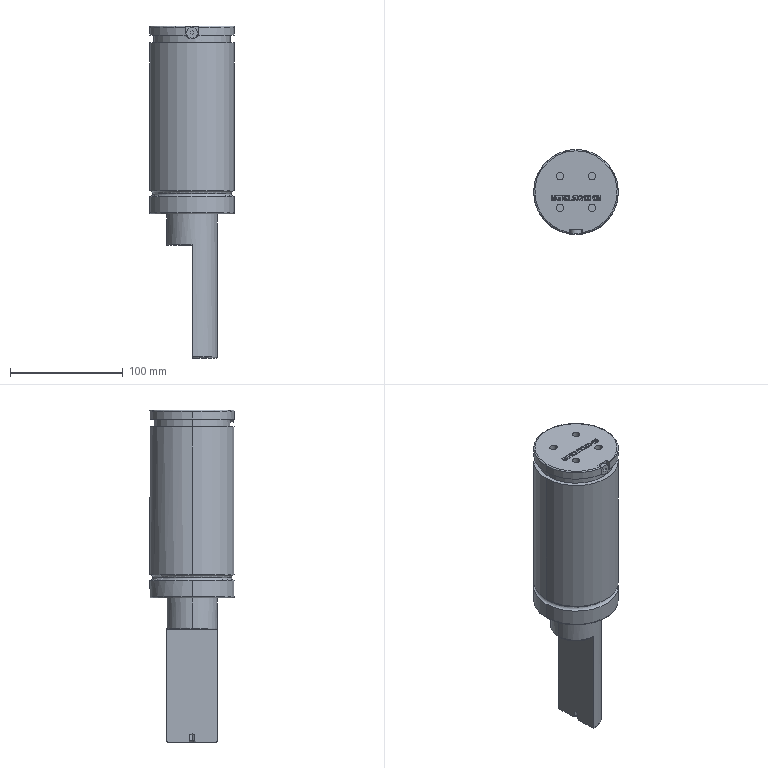Part | STEP file | 1_id2330_x_t | 1 solid | 228 faces | box 75.2 x 75.2 x 295 mm | volume 855529 mm3 | plane 154 | other 34 | cylinder 26 | cone 8 | torus 6 | commonest cylinder face diameters 6.6 x8 75.2 x7 4.9 x4 9.5 x2 45 x2 67.6 x2